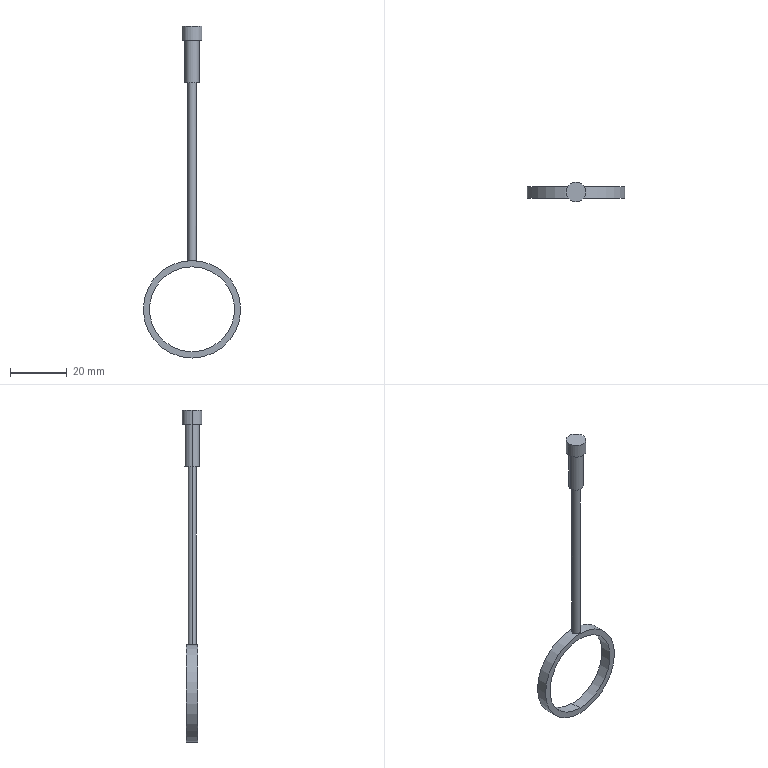Part | STEP file | Resist_ncia- reg. - A | 1 solid | 15 faces | box 34.4 x 7 x 117.2 mm | volume 1821 mm3 | cylinder 10 | plane 5 | commonest cylinder face diameters 3 x2 5 x2 7 x2 30 x2 34.4 x2
STEP:
#1=CARTESIAN_POINT('',(0.,0.,0.));
#2=DIRECTION('',(0.,0.,1.));
#3=DIRECTION('',(1.,0.,0.));
#4=AXIS2_PLACEMENT_3D('',#1,#2,#3);
#5=CARTESIAN_POINT('',(0.,-2.,-2.));
#6=VERTEX_POINT('',#5);
#7=CARTESIAN_POINT('',(0.,2.,-2.));
#8=VERTEX_POINT('',#7);
#9=CARTESIAN_POINT('',(0.,-2.,-2.));
#10=DIRECTION('',(0.,1.,0.));
#11=VECTOR('',#10,1.);
#12=LINE('',#9,#11);
#13=CARTESIAN_POINT('',(0.,-2.,-17.));
#14=DIRECTION('',(0.,1.,0.));
#15=DIRECTION('',(0.,0.,1.));
#16=AXIS2_PLACEMENT_3D('',#13,#14,#15);
#17=CYLINDRICAL_SURFACE('',#16,15.);
#18=CARTESIAN_POINT('',(6.283,0.));
#19=DIRECTION('',(0.,1.));
#20=VECTOR('',#19,1.);
#21=LINE('',#18,#20);
#22=(GEOMETRIC_REPRESENTATION_CONTEXT(2)PARAMETRIC_REPRESENTATION_CONTEXT()REPRESENTATION_CONTEXT('',''));
#23=DEFINITIONAL_REPRESENTATION('',(#21),#22);
#24=PCURVE('',#17,#23);
#25=CARTESIAN_POINT('',(0.,-2.,-17.));
#26=DIRECTION('',(0.,1.,0.));
#27=DIRECTION('',(0.,0.,1.));
#28=AXIS2_PLACEMENT_3D('',#25,#26,#27);
#29=CYLINDRICAL_SURFACE('',#28,15.);
#30=CARTESIAN_POINT('',(0.,0.));
#31=DIRECTION('',(0.,1.));
#32=VECTOR('',#31,1.);
#33=LINE('',#30,#32);
#34=(GEOMETRIC_REPRESENTATION_CONTEXT(2)PARAMETRIC_REPRESENTATION_CONTEXT()REPRESENTATION_CONTEXT('',''));
#35=DEFINITIONAL_REPRESENTATION('',(#33),#34);
#36=PCURVE('',#29,#35);
#37=SURFACE_CURVE('',#12,(#24,#36),.PCURVE_S1.);
#38=EDGE_CURVE('',#6,#8,#37,.T.);
#39=ORIENTED_EDGE('',*,*,#38,.T.);
#40=CARTESIAN_POINT('',(0.,2.,-32.));
#41=VERTEX_POINT('',#40);
#42=CARTESIAN_POINT('',(0.,2.,-17.));
#43=DIRECTION('',(0.,1.,0.));
#44=DIRECTION('',(0.,0.,1.));
#45=AXIS2_PLACEMENT_3D('',#42,#43,#44);
#46=CIRCLE('',#45,15.);
#47=CARTESIAN_POINT('',(0.,4.));
#48=DIRECTION('',(1.,0.));
#49=VECTOR('',#48,1.);
#50=LINE('',#47,#49);
#51=(GEOMETRIC_REPRESENTATION_CONTEXT(2)PARAMETRIC_REPRESENTATION_CONTEXT()REPRESENTATION_CONTEXT('',''));
#52=DEFINITIONAL_REPRESENTATION('',(#50),#51);
#53=PCURVE('',#17,#52);
#54=CARTESIAN_POINT('',(0.,2.,-17.));
#55=DIRECTION('',(0.,1.,0.));
#56=DIRECTION('',(0.,0.,1.));
#57=AXIS2_PLACEMENT_3D('',#54,#55,#56);
#58=PLANE('',#57);
#59=CARTESIAN_POINT('',(0.,0.));
#60=DIRECTION('',(1.,0.));
#61=AXIS2_PLACEMENT_2D('',#59,#60);
#62=CIRCLE('',#61,15.);
#63=(GEOMETRIC_REPRESENTATION_CONTEXT(2)PARAMETRIC_REPRESENTATION_CONTEXT()REPRESENTATION_CONTEXT('',''));
#64=DEFINITIONAL_REPRESENTATION('',(#62),#63);
#65=PCURVE('',#58,#64);
#66=SURFACE_CURVE('',#46,(#53,#65),.PCURVE_S1.);
#67=EDGE_CURVE('',#41,#8,#66,.T.);
#68=ORIENTED_EDGE('',*,*,#67,.F.);
#69=CARTESIAN_POINT('',(0.,-2.,-32.));
#70=VERTEX_POINT('',#69);
#71=CARTESIAN_POINT('',(0.,-2.,-32.));
#72=DIRECTION('',(0.,1.,0.));
#73=VECTOR('',#72,1.);
#74=LINE('',#71,#73);
#75=CARTESIAN_POINT('',(3.142,0.));
#76=DIRECTION('',(0.,1.));
#77=VECTOR('',#76,1.);
#78=LINE('',#75,#77);
#79=(GEOMETRIC_REPRESENTATION_CONTEXT(2)PARAMETRIC_REPRESENTATION_CONTEXT()REPRESENTATION_CONTEXT('',''));
#80=DEFINITIONAL_REPRESENTATION('',(#78),#79);
#81=PCURVE('',#17,#80);
#82=CARTESIAN_POINT('',(3.142,0.));
#83=DIRECTION('',(0.,1.));
#84=VECTOR('',#83,1.);
#85=LINE('',#82,#84);
#86=(GEOMETRIC_REPRESENTATION_CONTEXT(2)PARAMETRIC_REPRESENTATION_CONTEXT()REPRESENTATION_CONTEXT('',''));
#87=DEFINITIONAL_REPRESENTATION('',(#85),#86);
#88=PCURVE('',#29,#87);
#89=SURFACE_CURVE('',#74,(#81,#88),.PCURVE_S1.);
#90=EDGE_CURVE('',#70,#41,#89,.T.);
#91=ORIENTED_EDGE('',*,*,#90,.F.);
#92=CARTESIAN_POINT('',(0.,-2.,-17.));
#93=DIRECTION('',(0.,1.,0.));
#94=DIRECTION('',(0.,0.,1.));
#95=AXIS2_PLACEMENT_3D('',#92,#93,#94);
#96=CIRCLE('',#95,15.);
#97=CARTESIAN_POINT('',(0.,0.));
#98=DIRECTION('',(1.,0.));
#99=VECTOR('',#98,1.);
#100=LINE('',#97,#99);
#101=(GEOMETRIC_REPRESENTATION_CONTEXT(2)PARAMETRIC_REPRESENTATION_CONTEXT()REPRESENTATION_CONTEXT('',''));
#102=DEFINITIONAL_REPRESENTATION('',(#100),#101);
#103=PCURVE('',#17,#102);
#104=CARTESIAN_POINT('',(0.,-2.,-17.));
#105=DIRECTION('',(0.,1.,0.));
#106=DIRECTION('',(0.,0.,1.));
#107=AXIS2_PLACEMENT_3D('',#104,#105,#106);
#108=PLANE('',#107);
#109=CARTESIAN_POINT('',(0.,0.));
#110=DIRECTION('',(1.,0.));
#111=AXIS2_PLACEMENT_2D('',#109,#110);
#112=CIRCLE('',#111,15.);
#113=(GEOMETRIC_REPRESENTATION_CONTEXT(2)PARAMETRIC_REPRESENTATION_CONTEXT()REPRESENTATION_CONTEXT('',''));
#114=DEFINITIONAL_REPRESENTATION('',(#112),#113);
#115=PCURVE('',#108,#114);
#116=SURFACE_CURVE('',#96,(#103,#115),.PCURVE_S1.);
#117=EDGE_CURVE('',#70,#6,#116,.T.);
#118=ORIENTED_EDGE('',*,*,#117,.T.);
#119=EDGE_LOOP('',(#39,#68,#91,#118));
#120=FACE_BOUND('',#119,.F.);
#121=ADVANCED_FACE('',(#120),#17,.F.);
#122=CARTESIAN_POINT('',(0.,-2.,0.2));
#123=VERTEX_POINT('',#122);
#124=CARTESIAN_POINT('',(0.,-2.,-34.2));
#125=VERTEX_POINT('',#124);
#126=CARTESIAN_POINT('',(0.,-2.,-17.));
#127=DIRECTION('',(0.,1.,0.));
#128=DIRECTION('',(0.,0.,1.));
#129=AXIS2_PLACEMENT_3D('',#126,#127,#128);
#130=CIRCLE('',#129,17.2);
#131=CARTESIAN_POINT('',(0.,-2.,-17.));
#132=DIRECTION('',(0.,1.,0.));
#133=DIRECTION('',(0.,0.,1.));
#134=AXIS2_PLACEMENT_3D('',#131,#132,#133);
#135=CYLINDRICAL_SURFACE('',#134,17.2);
#136=CARTESIAN_POINT('',(0.,0.));
#137=DIRECTION('',(1.,0.));
#138=VECTOR('',#137,1.);
#139=LINE('',#136,#138);
#140=(GEOMETRIC_REPRESENTATION_CONTEXT(2)PARAMETRIC_REPRESENTATION_CONTEXT()REPRESENTATION_CONTEXT('',''));
#141=DEFINITIONAL_REPRESENTATION('',(#139),#140);
#142=PCURVE('',#135,#141);
#143=CARTESIAN_POINT('',(0.,0.));
#144=DIRECTION('',(1.,0.));
#145=AXIS2_PLACEMENT_2D('',#143,#144);
#146=CIRCLE('',#145,17.2);
#147=(GEOMETRIC_REPRESENTATION_CONTEXT(2)PARAMETRIC_REPRESENTATION_CONTEXT()REPRESENTATION_CONTEXT('',''));
#148=DEFINITIONAL_REPRESENTATION('',(#146),#147);
#149=PCURVE('',#108,#148);
#150=SURFACE_CURVE('',#130,(#142,#149),.PCURVE_S1.);
#151=EDGE_CURVE('',#123,#125,#150,.T.);
#152=ORIENTED_EDGE('',*,*,#151,.T.);
#153=CARTESIAN_POINT('',(0.,2.,-34.2));
#154=VERTEX_POINT('',#153);
#155=CARTESIAN_POINT('',(0.,-2.,-34.2));
#156=DIRECTION('',(0.,1.,0.));
#157=VECTOR('',#156,1.);
#158=LINE('',#155,#157);
#159=CARTESIAN_POINT('',(3.142,0.));
#160=DIRECTION('',(0.,1.));
#161=VECTOR('',#160,1.);
#162=LINE('',#159,#161);
#163=(GEOMETRIC_REPRESENTATION_CONTEXT(2)PARAMETRIC_REPRESENTATION_CONTEXT()REPRESENTATION_CONTEXT('',''));
#164=DEFINITIONAL_REPRESENTATION('',(#162),#163);
#165=PCURVE('',#135,#164);
#166=CARTESIAN_POINT('',(0.,-2.,-17.));
#167=DIRECTION('',(0.,1.,0.));
#168=DIRECTION('',(0.,0.,1.));
#169=AXIS2_PLACEMENT_3D('',#166,#167,#168);
#170=CYLINDRICAL_SURFACE('',#169,17.2);
#171=CARTESIAN_POINT('',(3.142,0.));
#172=DIRECTION('',(0.,1.));
#173=VECTOR('',#172,1.);
#174=LINE('',#171,#173);
#175=(GEOMETRIC_REPRESENTATION_CONTEXT(2)PARAMETRIC_REPRESENTATION_CONTEXT()REPRESENTATION_CONTEXT('',''));
#176=DEFINITIONAL_REPRESENTATION('',(#174),#175);
#177=PCURVE('',#170,#176);
#178=SURFACE_CURVE('',#158,(#165,#177),.PCURVE_S1.);
#179=EDGE_CURVE('',#125,#154,#178,.T.);
#180=ORIENTED_EDGE('',*,*,#179,.T.);
#181=CARTESIAN_POINT('',(0.,2.,0.2));
#182=VERTEX_POINT('',#181);
#183=CARTESIAN_POINT('',(0.,2.,-17.));
#184=DIRECTION('',(0.,1.,0.));
#185=DIRECTION('',(0.,0.,1.));
#186=AXIS2_PLACEMENT_3D('',#183,#184,#185);
#187=CIRCLE('',#186,17.2);
#188=CARTESIAN_POINT('',(0.,4.));
#189=DIRECTION('',(1.,0.));
#190=VECTOR('',#189,1.);
#191=LINE('',#188,#190);
#192=(GEOMETRIC_REPRESENTATION_CONTEXT(2)PARAMETRIC_REPRESENTATION_CONTEXT()REPRESENTATION_CONTEXT('',''));
#193=DEFINITIONAL_REPRESENTATION('',(#191),#192);
#194=PCURVE('',#135,#193);
#195=CARTESIAN_POINT('',(0.,0.));
#196=DIRECTION('',(1.,0.));
#197=AXIS2_PLACEMENT_2D('',#195,#196);
#198=CIRCLE('',#197,17.2);
#199=(GEOMETRIC_REPRESENTATION_CONTEXT(2)PARAMETRIC_REPRESENTATION_CONTEXT()REPRESENTATION_CONTEXT('',''));
#200=DEFINITIONAL_REPRESENTATION('',(#198),#199);
#201=PCURVE('',#58,#200);
#202=SURFACE_CURVE('',#187,(#194,#201),.PCURVE_S1.);
#203=EDGE_CURVE('',#182,#154,#202,.T.);
#204=ORIENTED_EDGE('',*,*,#203,.F.);
#205=CARTESIAN_POINT('',(0.,1.5,0.2));
#206=VERTEX_POINT('',#205);
#207=CARTESIAN_POINT('',(0.,-2.,0.2));
#208=DIRECTION('',(0.,1.,0.));
#209=VECTOR('',#208,1.);
#210=LINE('',#207,#209);
#211=CARTESIAN_POINT('',(0.,0.));
#212=DIRECTION('',(0.,1.));
#213=VECTOR('',#212,1.);
#214=LINE('',#211,#213);
#215=(GEOMETRIC_REPRESENTATION_CONTEXT(2)PARAMETRIC_REPRESENTATION_CONTEXT()REPRESENTATION_CONTEXT('',''));
#216=DEFINITIONAL_REPRESENTATION('',(#214),#215);
#217=PCURVE('',#135,#216);
#218=CARTESIAN_POINT('',(6.283,0.));
#219=DIRECTION('',(0.,1.));
#220=VECTOR('',#219,1.);
#221=LINE('',#218,#220);
#222=(GEOMETRIC_REPRESENTATION_CONTEXT(2)PARAMETRIC_REPRESENTATION_CONTEXT()REPRESENTATION_CONTEXT('',''));
#223=DEFINITIONAL_REPRESENTATION('',(#221),#222);
#224=PCURVE('',#170,#223);
#225=SURFACE_CURVE('',#210,(#217,#224),.PCURVE_S1.);
#226=EDGE_CURVE('',#206,#182,#225,.T.);
#227=ORIENTED_EDGE('',*,*,#226,.F.);
#228=CARTESIAN_POINT('',(1.5,0.,0.1345));
#229=VERTEX_POINT('',#228);
#230=CARTESIAN_POINT('',(1.5,0.,0.1345));
#231=CARTESIAN_POINT('',(1.5,0.1959,0.1345));
#232=CARTESIAN_POINT('',(1.461,0.3934,0.138));
#233=CARTESIAN_POINT('',(1.311,0.7546,0.1501));
#234=CARTESIAN_POINT('',(1.199,0.922,0.1587));
#235=CARTESIAN_POINT('',(0.9918,1.13,0.1715));
#236=CARTESIAN_POINT('',(0.9147,1.193,0.1759));
#237=CARTESIAN_POINT('',(0.7516,1.302,0.1838));
#238=CARTESIAN_POINT('',(0.6654,1.348,0.1874));
#239=CARTESIAN_POINT('',(0.4838,1.423,0.1934));
#240=CARTESIAN_POINT('',(0.3884,1.452,0.1959));
#241=CARTESIAN_POINT('',(0.1966,1.49,0.1991));
#242=CARTESIAN_POINT('',(0.09911,1.5,0.2));
#243=CARTESIAN_POINT('',(0.,1.5,0.2));
#244=B_SPLINE_CURVE_WITH_KNOTS('',3,(#230,#231,#232,#233,#234,#235,#236,#237,#238,#239,#240,#241,#242,#243),.UNSPECIFIED.,.F.,.F.,(4,2,2,2,2,2,4),(0.004692,0.005279,0.005865,0.006159,0.006452,0.006745,0.007038),.UNSPECIFIED.);
#245=CARTESIAN_POINT('',(0.08732,2.));
#246=CARTESIAN_POINT('',(0.08732,2.018));
#247=CARTESIAN_POINT('',(0.08728,2.053));
#248=CARTESIAN_POINT('',(0.08711,2.107));
#249=CARTESIAN_POINT('',(0.08683,2.16));
#250=CARTESIAN_POINT('',(0.08644,2.213));
#251=CARTESIAN_POINT('',(0.08594,2.266));
#252=CARTESIAN_POINT('',(0.08532,2.319));
#253=CARTESIAN_POINT('',(0.08461,2.371));
#254=CARTESIAN_POINT('',(0.08378,2.423));
#255=CARTESIAN_POINT('',(0.08285,2.474));
#256=CARTESIAN_POINT('',(0.08182,2.524));
#257=CARTESIAN_POINT('',(0.08068,2.574));
#258=CARTESIAN_POINT('',(0.07943,2.623));
#259=CARTESIAN_POINT('',(0.07809,2.671));
#260=CARTESIAN_POINT('',(0.07664,2.719));
#261=CARTESIAN_POINT('',(0.07509,2.765));
#262=CARTESIAN_POINT('',(0.07345,2.811));
#263=CARTESIAN_POINT('',(0.07171,2.855));
#264=CARTESIAN_POINT('',(0.06989,2.899));
#265=CARTESIAN_POINT('',(0.06797,2.941));
#266=CARTESIAN_POINT('',(0.06598,2.982));
#267=CARTESIAN_POINT('',(0.0639,3.022));
#268=CARTESIAN_POINT('',(0.06174,3.061));
#269=CARTESIAN_POINT('',(0.0595,3.098));
#270=CARTESIAN_POINT('',(0.05717,3.134));
#271=CARTESIAN_POINT('',(0.05476,3.168));
#272=CARTESIAN_POINT('',(0.05229,3.201));
#273=CARTESIAN_POINT('',(0.04975,3.233));
#274=CARTESIAN_POINT('',(0.04716,3.262));
#275=CARTESIAN_POINT('',(0.04452,3.29));
#276=CARTESIAN_POINT('',(0.04183,3.317));
#277=CARTESIAN_POINT('',(0.03908,3.341));
#278=CARTESIAN_POINT('',(0.03628,3.364));
#279=CARTESIAN_POINT('',(0.03342,3.386));
#280=CARTESIAN_POINT('',(0.03052,3.406));
#281=CARTESIAN_POINT('',(0.02756,3.423));
#282=CARTESIAN_POINT('',(0.02458,3.44));
#283=CARTESIAN_POINT('',(0.02156,3.454));
#284=CARTESIAN_POINT('',(0.01853,3.466));
#285=CARTESIAN_POINT('',(0.01549,3.476));
#286=CARTESIAN_POINT('',(0.01243,3.485));
#287=CARTESIAN_POINT('',(0.009348,3.492));
#288=CARTESIAN_POINT('',(0.006252,3.496));
#289=CARTESIAN_POINT('',(0.003137,3.499));
#290=CARTESIAN_POINT('',(0.001048,3.5));
#291=CARTESIAN_POINT('',(0.,3.5));
#292=B_SPLINE_CURVE_WITH_KNOTS('',3,(#245,#246,#247,#248,#249,#250,#251,#252,#253,#254,#255,#256,#257,#258,#259,#260,#261,#262,#263,#264,#265,#266,#267,#268,#269,#270,#271,#272,#273,#274,#275,#276,#277,#278,#279,#280,#281,#282,#283,#284,#285,#286,#287,#288,#289,#290,#291),.UNSPECIFIED.,.F.,.F.,(4,1,1,1,1,1,1,1,1,1,1,1,1,1,1,1,1,1,1,1,1,1,1,1,1,1,1,1,1,1,1,1,1,1,1,1,1,1,1,1,1,1,1,1,4),(0.004692,0.004745,0.004799,0.004852,0.004905,0.004959,0.005012,0.005065,0.005119,0.005172,0.005225,0.005279,0.005332,0.005385,0.005439,0.005492,0.005545,0.005599,0.005652,0.005705,0.005759,0.005812,0.005865,0.005919,0.005972,0.006025,0.006079,0.006132,0.006185,0.006239,0.006292,0.006345,0.006399,0.006452,0.006505,0.006559,0.006612,0.006665,0.006718,0.006772,0.006825,0.006878,0.006932,0.006985,0.007038),.QUASI_UNIFORM_KNOTS.);
#293=(GEOMETRIC_REPRESENTATION_CONTEXT(2)PARAMETRIC_REPRESENTATION_CONTEXT()REPRESENTATION_CONTEXT('',''));
#294=DEFINITIONAL_REPRESENTATION('',(#292),#293);
#295=PCURVE('',#135,#294);
#296=CARTESIAN_POINT('',(0.,0.,63.));
#297=DIRECTION('',(0.,0.,-1.));
#298=DIRECTION('',(-1.,0.,0.));
#299=AXIS2_PLACEMENT_3D('',#296,#297,#298);
#300=CYLINDRICAL_SURFACE('',#299,1.5);
#301=CARTESIAN_POINT('',(3.142,62.866));
#302=CARTESIAN_POINT('',(3.13,62.866));
#303=CARTESIAN_POINT('',(3.106,62.865));
#304=CARTESIAN_POINT('',(3.07,62.865));
#305=CARTESIAN_POINT('',(3.035,62.865));
#306=CARTESIAN_POINT('',(2.999,62.864));
#307=CARTESIAN_POINT('',(2.963,62.863));
#308=CARTESIAN_POINT('',(2.927,62.863));
#309=CARTESIAN_POINT('',(2.892,62.862));
#310=CARTESIAN_POINT('',(2.856,62.86));
#311=CARTESIAN_POINT('',(2.82,62.859));
#312=CARTESIAN_POINT('',(2.784,62.858));
#313=CARTESIAN_POINT('',(2.749,62.856));
#314=CARTESIAN_POINT('',(2.713,62.854));
#315=CARTESIAN_POINT('',(2.678,62.852));
#316=CARTESIAN_POINT('',(2.642,62.85));
#317=CARTESIAN_POINT('',(2.606,62.848));
#318=CARTESIAN_POINT('',(2.571,62.846));
#319=CARTESIAN_POINT('',(2.535,62.844));
#320=CARTESIAN_POINT('',(2.499,62.842));
#321=CARTESIAN_POINT('',(2.463,62.84));
#322=CARTESIAN_POINT('',(2.428,62.837));
#323=CARTESIAN_POINT('',(2.392,62.835));
#324=CARTESIAN_POINT('',(2.357,62.833));
#325=CARTESIAN_POINT('',(2.321,62.83));
#326=CARTESIAN_POINT('',(2.285,62.828));
#327=CARTESIAN_POINT('',(2.249,62.826));
#328=CARTESIAN_POINT('',(2.213,62.823));
#329=CARTESIAN_POINT('',(2.177,62.821));
#330=CARTESIAN_POINT('',(2.142,62.819));
#331=CARTESIAN_POINT('',(2.106,62.817));
#332=CARTESIAN_POINT('',(2.071,62.815));
#333=CARTESIAN_POINT('',(2.035,62.813));
#334=CARTESIAN_POINT('',(2.,62.811));
#335=CARTESIAN_POINT('',(1.964,62.81));
#336=CARTESIAN_POINT('',(1.928,62.808));
#337=CARTESIAN_POINT('',(1.892,62.807));
#338=CARTESIAN_POINT('',(1.856,62.805));
#339=CARTESIAN_POINT('',(1.821,62.804));
#340=CARTESIAN_POINT('',(1.785,62.803));
#341=CARTESIAN_POINT('',(1.749,62.802));
#342=CARTESIAN_POINT('',(1.714,62.801));
#343=CARTESIAN_POINT('',(1.678,62.801));
#344=CARTESIAN_POINT('',(1.643,62.8));
#345=CARTESIAN_POINT('',(1.607,62.8));
#346=CARTESIAN_POINT('',(1.583,62.8));
#347=CARTESIAN_POINT('',(1.571,62.8));
#348=B_SPLINE_CURVE_WITH_KNOTS('',3,(#301,#302,#303,#304,#305,#306,#307,#308,#309,#310,#311,#312,#313,#314,#315,#316,#317,#318,#319,#320,#321,#322,#323,#324,#325,#326,#327,#328,#329,#330,#331,#332,#333,#334,#335,#336,#337,#338,#339,#340,#341,#342,#343,#344,#345,#346,#347),.UNSPECIFIED.,.F.,.F.,(4,1,1,1,1,1,1,1,1,1,1,1,1,1,1,1,1,1,1,1,1,1,1,1,1,1,1,1,1,1,1,1,1,1,1,1,1,1,1,1,1,1,1,1,4),(0.004692,0.004745,0.004799,0.004852,0.004905,0.004959,0.005012,0.005065,0.005119,0.005172,0.005225,0.005279,0.005332,0.005385,0.005439,0.005492,0.005545,0.005599,0.005652,0.005705,0.005759,0.005812,0.005865,0.005919,0.005972,0.006025,0.006079,0.006132,0.006185,0.006239,0.006292,0.006345,0.006399,0.006452,0.006505,0.006559,0.006612,0.006665,0.006718,0.006772,0.006825,0.006878,0.006932,0.006985,0.007038),.QUASI_UNIFORM_KNOTS.);
#349=(GEOMETRIC_REPRESENTATION_CONTEXT(2)PARAMETRIC_REPRESENTATION_CONTEXT()REPRESENTATION_CONTEXT('',''));
#350=DEFINITIONAL_REPRESENTATION('',(#348),#349);
#351=PCURVE('',#300,#350);
#352=SURFACE_CURVE('',#244,(#295,#351),.PCURVE_S1.);
#353=EDGE_CURVE('',#229,#206,#352,.T.);
#354=ORIENTED_EDGE('',*,*,#353,.F.);
#355=CARTESIAN_POINT('',(0.,-1.5,0.2));
#356=VERTEX_POINT('',#355);
#357=CARTESIAN_POINT('',(0.,-1.5,0.2));
#358=CARTESIAN_POINT('',(0.09787,-1.5,0.2));
#359=CARTESIAN_POINT('',(0.1973,-1.49,0.1991));
#360=CARTESIAN_POINT('',(0.3896,-1.452,0.1959));
#361=CARTESIAN_POINT('',(0.4831,-1.423,0.1935));
#362=CARTESIAN_POINT('',(0.6648,-1.348,0.1874));
#363=CARTESIAN_POINT('',(0.7525,-1.301,0.1837));
#364=CARTESIAN_POINT('',(0.9149,-1.193,0.1758));
#365=CARTESIAN_POINT('',(0.9907,-1.131,0.1716));
#366=CARTESIAN_POINT('',(1.131,-0.9906,0.1629));
#367=CARTESIAN_POINT('',(1.193,-0.9149,0.1587));
#368=CARTESIAN_POINT('',(1.301,-0.7525,0.1508));
#369=CARTESIAN_POINT('',(1.348,-0.6648,0.1471));
#370=CARTESIAN_POINT('',(1.423,-0.4831,0.141));
#371=CARTESIAN_POINT('',(1.452,-0.3896,0.1386));
#372=CARTESIAN_POINT('',(1.49,-0.1973,0.1353));
#373=CARTESIAN_POINT('',(1.5,-0.0979,0.1345));
#374=CARTESIAN_POINT('',(1.5,0.,0.1345));
#375=B_SPLINE_CURVE_WITH_KNOTS('',3,(#357,#358,#359,#360,#361,#362,#363,#364,#365,#366,#367,#368,#369,#370,#371,#372,#373,#374),.UNSPECIFIED.,.F.,.F.,(4,2,2,2,2,2,2,2,4),(0.002346,0.00264,0.002933,0.003226,0.003519,0.003812,0.004106,0.004399,0.004692),.UNSPECIFIED.);
#376=CARTESIAN_POINT('',(0.,0.5));
#377=CARTESIAN_POINT('',(0.001035,0.5));
#378=CARTESIAN_POINT('',(0.00311,0.5006));
#379=CARTESIAN_POINT('',(0.00623,0.5035));
#380=CARTESIAN_POINT('',(0.009348,0.5084));
#381=CARTESIAN_POINT('',(0.01245,0.5151));
#382=CARTESIAN_POINT('',(0.01554,0.5237));
#383=CARTESIAN_POINT('',(0.01859,0.5341));
#384=CARTESIAN_POINT('',(0.02161,0.5464));
#385=CARTESIAN_POINT('',(0.0246,0.5605));
#386=CARTESIAN_POINT('',(0.02756,0.5765));
#387=CARTESIAN_POINT('',(0.03048,0.5942));
#388=CARTESIAN_POINT('',(0.03338,0.6138));
#389=CARTESIAN_POINT('',(0.03624,0.6353));
#390=CARTESIAN_POINT('',(0.03907,0.6585));
#391=CARTESIAN_POINT('',(0.04184,0.6834));
#392=CARTESIAN_POINT('',(0.04455,0.71));
#393=CARTESIAN_POINT('',(0.0472,0.7382));
#394=CARTESIAN_POINT('',(0.04978,0.7678));
#395=CARTESIAN_POINT('',(0.0523,0.7989));
#396=CARTESIAN_POINT('',(0.05475,0.8316));
#397=CARTESIAN_POINT('',(0.05714,0.8659));
#398=CARTESIAN_POINT('',(0.05946,0.9017));
#399=CARTESIAN_POINT('',(0.06172,0.9391));
#400=CARTESIAN_POINT('',(0.0639,0.9779));
#401=CARTESIAN_POINT('',(0.06599,1.018));
#402=CARTESIAN_POINT('',(0.06798,1.059));
#403=CARTESIAN_POINT('',(0.06989,1.101));
#404=CARTESIAN_POINT('',(0.0717,1.144));
#405=CARTESIAN_POINT('',(0.07343,1.188));
#406=CARTESIAN_POINT('',(0.07507,1.234));
#407=CARTESIAN_POINT('',(0.07662,1.281));
#408=CARTESIAN_POINT('',(0.07807,1.328));
#409=CARTESIAN_POINT('',(0.07943,1.377));
#410=CARTESIAN_POINT('',(0.08068,1.426));
#411=CARTESIAN_POINT('',(0.08182,1.476));
#412=CARTESIAN_POINT('',(0.08286,1.526));
#413=CARTESIAN_POINT('',(0.08379,1.577));
#414=CARTESIAN_POINT('',(0.08461,1.628));
#415=CARTESIAN_POINT('',(0.08533,1.68));
#416=CARTESIAN_POINT('',(0.08594,1.733));
#417=CARTESIAN_POINT('',(0.08644,1.786));
#418=CARTESIAN_POINT('',(0.08683,1.839));
#419=CARTESIAN_POINT('',(0.08711,1.893));
#420=CARTESIAN_POINT('',(0.08728,1.946));
#421=CARTESIAN_POINT('',(0.08732,1.982));
#422=CARTESIAN_POINT('',(0.08732,2.));
#423=B_SPLINE_CURVE_WITH_KNOTS('',3,(#376,#377,#378,#379,#380,#381,#382,#383,#384,#385,#386,#387,#388,#389,#390,#391,#392,#393,#394,#395,#396,#397,#398,#399,#400,#401,#402,#403,#404,#405,#406,#407,#408,#409,#410,#411,#412,#413,#414,#415,#416,#417,#418,#419,#420,#421,#422),.UNSPECIFIED.,.F.,.F.,(4,1,1,1,1,1,1,1,1,1,1,1,1,1,1,1,1,1,1,1,1,1,1,1,1,1,1,1,1,1,1,1,1,1,1,1,1,1,1,1,1,1,1,1,4),(0.002346,0.0024,0.002453,0.002506,0.00256,0.002613,0.002666,0.00272,0.002773,0.002826,0.00288,0.002933,0.002986,0.003039,0.003093,0.003146,0.003199,0.003253,0.003306,0.003359,0.003413,0.003466,0.003519,0.003573,0.003626,0.003679,0.003732,0.003786,0.003839,0.003892,0.003946,0.003999,0.004052,0.004106,0.004159,0.004212,0.004265,0.004319,0.004372,0.004425,0.004479,0.004532,0.004585,0.004639,0.004692),.QUASI_UNIFORM_KNOTS.);
#424=(GEOMETRIC_REPRESENTATION_CONTEXT(2)PARAMETRIC_REPRESENTATION_CONTEXT()REPRESENTATION_CONTEXT('',''));
#425=DEFINITIONAL_REPRESENTATION('',(#423),#424);
#426=PCURVE('',#135,#425);
#427=CARTESIAN_POINT('',(0.,0.,63.));
#428=DIRECTION('',(0.,0.,-1.));
#429=DIRECTION('',(-1.,0.,0.));
#430=AXIS2_PLACEMENT_3D('',#427,#428,#429);
#431=CYLINDRICAL_SURFACE('',#430,1.5);
#432=CARTESIAN_POINT('',(4.712,62.8));
#433=CARTESIAN_POINT('',(4.701,62.8));
#434=CARTESIAN_POINT('',(4.677,62.8));
#435=CARTESIAN_POINT('',(4.641,62.8));
#436=CARTESIAN_POINT('',(4.605,62.801));
#437=CARTESIAN_POINT('',(4.569,62.801));
#438=CARTESIAN_POINT('',(4.533,62.802));
#439=CARTESIAN_POINT('',(4.498,62.803));
#440=CARTESIAN_POINT('',(4.462,62.804));
#441=CARTESIAN_POINT('',(4.427,62.805));
#442=CARTESIAN_POINT('',(4.391,62.807));
#443=CARTESIAN_POINT('',(4.355,62.808));
#444=CARTESIAN_POINT('',(4.32,62.81));
#445=CARTESIAN_POINT('',(4.284,62.811));
#446=CARTESIAN_POINT('',(4.248,62.813));
#447=CARTESIAN_POINT('',(4.212,62.815));
#448=CARTESIAN_POINT('',(4.176,62.817));
#449=CARTESIAN_POINT('',(4.141,62.819));
#450=CARTESIAN_POINT('',(4.105,62.821));
#451=CARTESIAN_POINT('',(4.07,62.823));
#452=CARTESIAN_POINT('',(4.034,62.826));
#453=CARTESIAN_POINT('',(3.999,62.828));
#454=CARTESIAN_POINT('',(3.963,62.83));
#455=CARTESIAN_POINT('',(3.927,62.833));
#456=CARTESIAN_POINT('',(3.891,62.835));
#457=CARTESIAN_POINT('',(3.855,62.837));
#458=CARTESIAN_POINT('',(3.82,62.84));
#459=CARTESIAN_POINT('',(3.784,62.842));
#460=CARTESIAN_POINT('',(3.749,62.844));
#461=CARTESIAN_POINT('',(3.713,62.846));
#462=CARTESIAN_POINT('',(3.677,62.848));
#463=CARTESIAN_POINT('',(3.642,62.85));
#464=CARTESIAN_POINT('',(3.606,62.852));
#465=CARTESIAN_POINT('',(3.57,62.854));
#466=CARTESIAN_POINT('',(3.534,62.856));
#467=CARTESIAN_POINT('',(3.499,62.858));
#468=CARTESIAN_POINT('',(3.463,62.859));
#469=CARTESIAN_POINT('',(3.427,62.86));
#470=CARTESIAN_POINT('',(3.392,62.862));
#471=CARTESIAN_POINT('',(3.356,62.863));
#472=CARTESIAN_POINT('',(3.321,62.863));
#473=CARTESIAN_POINT('',(3.285,62.864));
#474=CARTESIAN_POINT('',(3.249,62.865));
#475=CARTESIAN_POINT('',(3.213,62.865));
#476=CARTESIAN_POINT('',(3.177,62.865));
#477=CARTESIAN_POINT('',(3.153,62.866));
#478=CARTESIAN_POINT('',(3.142,62.866));
#479=B_SPLINE_CURVE_WITH_KNOTS('',3,(#432,#433,#434,#435,#436,#437,#438,#439,#440,#441,#442,#443,#444,#445,#446,#447,#448,#449,#450,#451,#452,#453,#454,#455,#456,#457,#458,#459,#460,#461,#462,#463,#464,#465,#466,#467,#468,#469,#470,#471,#472,#473,#474,#475,#476,#477,#478),.UNSPECIFIED.,.F.,.F.,(4,1,1,1,1,1,1,1,1,1,1,1,1,1,1,1,1,1,1,1,1,1,1,1,1,1,1,1,1,1,1,1,1,1,1,1,1,1,1,1,1,1,1,1,4),(0.002346,0.0024,0.002453,0.002506,0.00256,0.002613,0.002666,0.00272,0.002773,0.002826,0.00288,0.002933,0.002986,0.003039,0.003093,0.003146,0.003199,0.003253,0.003306,0.003359,0.003413,0.003466,0.003519,0.003573,0.003626,0.003679,0.003732,0.003786,0.003839,0.003892,0.003946,0.003999,0.004052,0.004106,0.004159,0.004212,0.004265,0.004319,0.004372,0.004425,0.004479,0.004532,0.004585,0.004639,0.004692),.QUASI_UNIFORM_KNOTS.);
#480=(GEOMETRIC_REPRESENTATION_CONTEXT(2)PARAMETRIC_REPRESENTATION_CONTEXT()REPRESENTATION_CONTEXT('',''));
#481=DEFINITIONAL_REPRESENTATION('',(#479),#480);
#482=PCURVE('',#431,#481);
#483=SURFACE_CURVE('',#375,(#426,#482),.PCURVE_S1.);
#484=EDGE_CURVE('',#356,#229,#483,.T.);
#485=ORIENTED_EDGE('',*,*,#484,.F.);
#486=CARTESIAN_POINT('',(0.,-2.,0.2));
#487=DIRECTION('',(0.,1.,0.));
#488=VECTOR('',#487,1.);
#489=LINE('',#486,#488);
#490=CARTESIAN_POINT('',(0.,0.));
#491=DIRECTION('',(0.,1.));
#492=VECTOR('',#491,1.);
#493=LINE('',#490,#492);
#494=(GEOMETRIC_REPRESENTATION_CONTEXT(2)PARAMETRIC_REPRESENTATION_CONTEXT()REPRESENTATION_CONTEXT('',''));
#495=DEFINITIONAL_REPRESENTATION('',(#493),#494);
#496=PCURVE('',#135,#495);
#497=CARTESIAN_POINT('',(6.283,0.));
#498=DIRECTION('',(0.,1.));
#499=VECTOR('',#498,1.);
#500=LINE('',#497,#499);
#501=(GEOMETRIC_REPRESENTATION_CONTEXT(2)PARAMETRIC_REPRESENTATION_CONTEXT()REPRESENTATION_CONTEXT('',''));
#502=DEFINITIONAL_REPRESENTATION('',(#500),#501);
#503=PCURVE('',#170,#502);
#504=SURFACE_CURVE('',#489,(#496,#503),.PCURVE_S1.);
#505=EDGE_CURVE('',#123,#356,#504,.T.);
#506=ORIENTED_EDGE('',*,*,#505,.F.);
#507=EDGE_LOOP('',(#152,#180,#204,#227,#354,#485,#506));
#508=FACE_BOUND('',#507,.T.);
#509=ADVANCED_FACE('',(#508),#135,.T.);
#510=CARTESIAN_POINT('',(3.5,0.,83.));
#511=VERTEX_POINT('',#510);
#512=CARTESIAN_POINT('',(-3.5,0.,83.));
#513=VERTEX_POINT('',#512);
#514=CARTESIAN_POINT('',(0.,0.,83.));
#515=DIRECTION('',(0.,0.,1.));
#516=DIRECTION('',(1.,0.,0.));
#517=AXIS2_PLACEMENT_3D('',#514,#515,#516);
#518=CIRCLE('',#517,3.5);
#519=CARTESIAN_POINT('',(0.,0.,83.));
#520=DIRECTION('',(0.,0.,-1.));
#521=DIRECTION('',(-1.,0.,0.));
#522=AXIS2_PLACEMENT_3D('',#519,#520,#521);
#523=CYLINDRICAL_SURFACE('',#522,3.5);
#524=CARTESIAN_POINT('',(3.142,0.));
#525=DIRECTION('',(-1.,0.));
#526=VECTOR('',#525,1.);
#527=LINE('',#524,#526);
#528=(GEOMETRIC_REPRESENTATION_CONTEXT(2)PARAMETRIC_REPRESENTATION_CONTEXT()REPRESENTATION_CONTEXT('',''));
#529=DEFINITIONAL_REPRESENTATION('',(#527),#528);
#530=PCURVE('',#523,#529);
#531=CARTESIAN_POINT('',(0.,0.,83.));
#532=DIRECTION('',(0.,0.,1.));
#533=DIRECTION('',(1.,0.,0.));
#534=AXIS2_PLACEMENT_3D('',#531,#532,#533);
#535=PLANE('',#534);
#536=CARTESIAN_POINT('',(0.,0.));
#537=DIRECTION('',(1.,0.));
#538=AXIS2_PLACEMENT_2D('',#536,#537);
#539=CIRCLE('',#538,3.5);
#540=(GEOMETRIC_REPRESENTATION_CONTEXT(2)PARAMETRIC_REPRESENTATION_CONTEXT()REPRESENTATION_CONTEXT('',''));
#541=DEFINITIONAL_REPRESENTATION('',(#539),#540);
#542=PCURVE('',#535,#541);
#543=SURFACE_CURVE('',#518,(#530,#542),.PCURVE_S1.);
#544=EDGE_CURVE('',#511,#513,#543,.T.);
#545=ORIENTED_EDGE('',*,*,#544,.F.);
#546=CARTESIAN_POINT('',(3.5,0.,78.));
#547=VERTEX_POINT('',#546);
#548=CARTESIAN_POINT('',(3.5,0.,83.));
#549=DIRECTION('',(0.,0.,-1.));
#550=VECTOR('',#549,1.);
#551=LINE('',#548,#550);
#552=CARTESIAN_POINT('',(3.142,0.));
#553=DIRECTION('',(0.,1.));
#554=VECTOR('',#553,1.);
#555=LINE('',#552,#554);
#556=(GEOMETRIC_REPRESENTATION_CONTEXT(2)PARAMETRIC_REPRESENTATION_CONTEXT()REPRESENTATION_CONTEXT('',''));
#557=DEFINITIONAL_REPRESENTATION('',(#555),#556);
#558=PCURVE('',#523,#557);
#559=CARTESIAN_POINT('',(0.,0.,83.));
#560=DIRECTION('',(0.,0.,-1.));
#561=DIRECTION('',(-1.,0.,0.));
#562=AXIS2_PLACEMENT_3D('',#559,#560,#561);
#563=CYLINDRICAL_SURFACE('',#562,3.5);
#564=CARTESIAN_POINT('',(3.142,0.));
#565=DIRECTION('',(0.,1.));
#566=VECTOR('',#565,1.);
#567=LINE('',#564,#566);
#568=(GEOMETRIC_REPRESENTATION_CONTEXT(2)PARAMETRIC_REPRESENTATION_CONTEXT()REPRESENTATION_CONTEXT('',''));
#569=DEFINITIONAL_REPRESENTATION('',(#567),#568);
#570=PCURVE('',#563,#569);
#571=SURFACE_CURVE('',#551,(#558,#570),.PCURVE_S1.);
#572=EDGE_CURVE('',#511,#547,#571,.T.);
#573=ORIENTED_EDGE('',*,*,#572,.T.);
#574=CARTESIAN_POINT('',(-3.5,0.,78.));
#575=VERTEX_POINT('',#574);
#576=CARTESIAN_POINT('',(0.,0.,78.));
#577=DIRECTION('',(0.,0.,1.));
#578=DIRECTION('',(1.,0.,0.));
#579=AXIS2_PLACEMENT_3D('',#576,#577,#578);
#580=CIRCLE('',#579,3.5);
#581=CARTESIAN_POINT('',(3.142,5.));
#582=DIRECTION('',(-1.,0.));
#583=VECTOR('',#582,1.);
#584=LINE('',#581,#583);
#585=(GEOMETRIC_REPRESENTATION_CONTEXT(2)PARAMETRIC_REPRESENTATION_CONTEXT()REPRESENTATION_CONTEXT('',''));
#586=DEFINITIONAL_REPRESENTATION('',(#584),#585);
#587=PCURVE('',#523,#586);
#588=CARTESIAN_POINT('',(0.,0.,78.));
#589=DIRECTION('',(0.,0.,1.));
#590=DIRECTION('',(1.,0.,0.));
#591=AXIS2_PLACEMENT_3D('',#588,#589,#590);
#592=PLANE('',#591);
#593=CARTESIAN_POINT('',(0.,0.));
#594=DIRECTION('',(1.,0.));
#595=AXIS2_PLACEMENT_2D('',#593,#594);
#596=CIRCLE('',#595,3.5);
#597=(GEOMETRIC_REPRESENTATION_CONTEXT(2)PARAMETRIC_REPRESENTATION_CONTEXT()REPRESENTATION_CONTEXT('',''));
#598=DEFINITIONAL_REPRESENTATION('',(#596),#597);
#599=PCURVE('',#592,#598);
#600=SURFACE_CURVE('',#580,(#587,#599),.PCURVE_S1.);
#601=EDGE_CURVE('',#547,#575,#600,.T.);
#602=ORIENTED_EDGE('',*,*,#601,.T.);
#603=CARTESIAN_POINT('',(-3.5,0.,83.));
#604=DIRECTION('',(0.,0.,-1.));
#605=VECTOR('',#604,1.);
#606=LINE('',#603,#605);
#607=CARTESIAN_POINT('',(0.,0.));
#608=DIRECTION('',(0.,1.));
#609=VECTOR('',#608,1.);
#610=LINE('',#607,#609);
#611=(GEOMETRIC_REPRESENTATION_CONTEXT(2)PARAMETRIC_REPRESENTATION_CONTEXT()REPRESENTATION_CONTEXT('',''));
#612=DEFINITIONAL_REPRESENTATION('',(#610),#611);
#613=PCURVE('',#523,#612);
#614=CARTESIAN_POINT('',(6.283,0.));
#615=DIRECTION('',(0.,1.));
#616=VECTOR('',#615,1.);
#617=LINE('',#614,#616);
#618=(GEOMETRIC_REPRESENTATION_CONTEXT(2)PARAMETRIC_REPRESENTATION_CONTEXT()REPRESENTATION_CONTEXT('',''));
#619=DEFINITIONAL_REPRESENTATION('',(#617),#618);
#620=PCURVE('',#563,#619);
#621=SURFACE_CURVE('',#606,(#613,#620),.PCURVE_S1.);
#622=EDGE_CURVE('',#513,#575,#621,.T.);
#623=ORIENTED_EDGE('',*,*,#622,.F.);
#624=EDGE_LOOP('',(#545,#573,#602,#623));
#625=FACE_BOUND('',#624,.T.);
#626=ADVANCED_FACE('',(#625),#523,.T.);
#627=CARTESIAN_POINT('',(2.5,0.,78.));
#628=VERTEX_POINT('',#627);
#629=CARTESIAN_POINT('',(-2.5,0.,78.));
#630=VERTEX_POINT('',#629);
#631=CARTESIAN_POINT('',(0.,0.,78.));
#632=DIRECTION('',(0.,0.,1.));
#633=DIRECTION('',(1.,0.,0.));
#634=AXIS2_PLACEMENT_3D('',#631,#632,#633);
#635=CIRCLE('',#634,2.5);
#636=CARTESIAN_POINT('',(0.,0.,78.));
#637=DIRECTION('',(0.,0.,-1.));
#638=DIRECTION('',(-1.,0.,0.));
#639=AXIS2_PLACEMENT_3D('',#636,#637,#638);
#640=CYLINDRICAL_SURFACE('',#639,2.5);
#641=CARTESIAN_POINT('',(3.142,0.));
#642=DIRECTION('',(-1.,0.));
#643=VECTOR('',#642,1.);
#644=LINE('',#641,#643);
#645=(GEOMETRIC_REPRESENTATION_CONTEXT(2)PARAMETRIC_REPRESENTATION_CONTEXT()REPRESENTATION_CONTEXT('',''));
#646=DEFINITIONAL_REPRESENTATION('',(#644),#645);
#647=PCURVE('',#640,#646);
#648=CARTESIAN_POINT('',(0.,0.));
#649=DIRECTION('',(1.,0.));
#650=AXIS2_PLACEMENT_2D('',#648,#649);
#651=CIRCLE('',#650,2.5);
#652=(GEOMETRIC_REPRESENTATION_CONTEXT(2)PARAMETRIC_REPRESENTATION_CONTEXT()REPRESENTATION_CONTEXT('',''));
#653=DEFINITIONAL_REPRESENTATION('',(#651),#652);
#654=PCURVE('',#592,#653);
#655=SURFACE_CURVE('',#635,(#647,#654),.PCURVE_S1.);
#656=EDGE_CURVE('',#628,#630,#655,.T.);
#657=ORIENTED_EDGE('',*,*,#656,.F.);
#658=CARTESIAN_POINT('',(2.5,0.,63.));
#659=VERTEX_POINT('',#658);
#660=CARTESIAN_POINT('',(2.5,0.,78.));
#661=DIRECTION('',(0.,0.,-1.));
#662=VECTOR('',#661,1.);
#663=LINE('',#660,#662);
#664=CARTESIAN_POINT('',(3.142,0.));
#665=DIRECTION('',(0.,1.));
#666=VECTOR('',#665,1.);
#667=LINE('',#664,#666);
#668=(GEOMETRIC_REPRESENTATION_CONTEXT(2)PARAMETRIC_REPRESENTATION_CONTEXT()REPRESENTATION_CONTEXT('',''));
#669=DEFINITIONAL_REPRESENTATION('',(#667),#668);
#670=PCURVE('',#640,#669);
#671=CARTESIAN_POINT('',(0.,0.,78.));
#672=DIRECTION('',(0.,0.,-1.));
#673=DIRECTION('',(-1.,0.,0.));
#674=AXIS2_PLACEMENT_3D('',#671,#672,#673);
#675=CYLINDRICAL_SURFACE('',#674,2.5);
#676=CARTESIAN_POINT('',(3.142,0.));
#677=DIRECTION('',(0.,1.));
#678=VECTOR('',#677,1.);
#679=LINE('',#676,#678);
#680=(GEOMETRIC_REPRESENTATION_CONTEXT(2)PARAMETRIC_REPRESENTATION_CONTEXT()REPRESENTATION_CONTEXT('',''));
#681=DEFINITIONAL_REPRESENTATION('',(#679),#680);
#682=PCURVE('',#675,#681);
#683=SURFACE_CURVE('',#663,(#670,#682),.PCURVE_S1.);
#684=EDGE_CURVE('',#628,#659,#683,.T.);
#685=ORIENTED_EDGE('',*,*,#684,.T.);
#686=CARTESIAN_POINT('',(-2.5,0.,63.));
#687=VERTEX_POINT('',#686);
#688=CARTESIAN_POINT('',(0.,0.,63.));
#689=DIRECTION('',(0.,0.,1.));
#690=DIRECTION('',(1.,0.,0.));
#691=AXIS2_PLACEMENT_3D('',#688,#689,#690);
#692=CIRCLE('',#691,2.5);
#693=CARTESIAN_POINT('',(3.142,15.));
#694=DIRECTION('',(-1.,0.));
#695=VECTOR('',#694,1.);
#696=LINE('',#693,#695);
#697=(GEOMETRIC_REPRESENTATION_CONTEXT(2)PARAMETRIC_REPRESENTATION_CONTEXT()REPRESENTATION_CONTEXT('',''));
#698=DEFINITIONAL_REPRESENTATION('',(#696),#697);
#699=PCURVE('',#640,#698);
#700=CARTESIAN_POINT('',(0.,0.,63.));
#701=DIRECTION('',(0.,0.,1.));
#702=DIRECTION('',(1.,0.,0.));
#703=AXIS2_PLACEMENT_3D('',#700,#701,#702);
#704=PLANE('',#703);
#705=CARTESIAN_POINT('',(0.,0.));
#706=DIRECTION('',(1.,0.));
#707=AXIS2_PLACEMENT_2D('',#705,#706);
#708=CIRCLE('',#707,2.5);
#709=(GEOMETRIC_REPRESENTATION_CONTEXT(2)PARAMETRIC_REPRESENTATION_CONTEXT()REPRESENTATION_CONTEXT('',''));
#710=DEFINITIONAL_REPRESENTATION('',(#708),#709);
#711=PCURVE('',#704,#710);
#712=SURFACE_CURVE('',#692,(#699,#711),.PCURVE_S1.);
#713=EDGE_CURVE('',#659,#687,#712,.T.);
#714=ORIENTED_EDGE('',*,*,#713,.T.);
#715=CARTESIAN_POINT('',(-2.5,0.,78.));
#716=DIRECTION('',(0.,0.,-1.));
#717=VECTOR('',#716,1.);
#718=LINE('',#715,#717);
#719=CARTESIAN_POINT('',(0.,0.));
#720=DIRECTION('',(0.,1.));
#721=VECTOR('',#720,1.);
#722=LINE('',#719,#721);
#723=(GEOMETRIC_REPRESENTATION_CONTEXT(2)PARAMETRIC_REPRESENTATION_CONTEXT()REPRESENTATION_CONTEXT('',''));
#724=DEFINITIONAL_REPRESENTATION('',(#722),#723);
#725=PCURVE('',#640,#724);
#726=CARTESIAN_POINT('',(6.283,0.));
#727=DIRECTION('',(0.,1.));
#728=VECTOR('',#727,1.);
#729=LINE('',#726,#728);
#730=(GEOMETRIC_REPRESENTATION_CONTEXT(2)PARAMETRIC_REPRESENTATION_CONTEXT()REPRESENTATION_CONTEXT('',''));
#731=DEFINITIONAL_REPRESENTATION('',(#729),#730);
#732=PCURVE('',#675,#731);
#733=SURFACE_CURVE('',#718,(#725,#732),.PCURVE_S1.);
#734=EDGE_CURVE('',#630,#687,#733,.T.);
#735=ORIENTED_EDGE('',*,*,#734,.F.);
#736=EDGE_LOOP('',(#657,#685,#714,#735));
#737=FACE_BOUND('',#736,.T.);
#738=ADVANCED_FACE('',(#737),#640,.T.);
#739=CARTESIAN_POINT('',(1.5,0.,63.));
#740=VERTEX_POINT('',#739);
#741=CARTESIAN_POINT('',(-1.5,0.,63.));
#742=VERTEX_POINT('',#741);
#743=CARTESIAN_POINT('',(0.,0.,63.));
#744=DIRECTION('',(0.,0.,1.));
#745=DIRECTION('',(1.,0.,0.));
#746=AXIS2_PLACEMENT_3D('',#743,#744,#745);
#747=CIRCLE('',#746,1.5);
#748=CARTESIAN_POINT('',(3.142,0.));
#749=DIRECTION('',(-1.,0.));
#750=VECTOR('',#749,1.);
#751=LINE('',#748,#750);
#752=(GEOMETRIC_REPRESENTATION_CONTEXT(2)PARAMETRIC_REPRESENTATION_CONTEXT()REPRESENTATION_CONTEXT('',''));
#753=DEFINITIONAL_REPRESENTATION('',(#751),#752);
#754=PCURVE('',#300,#753);
#755=CARTESIAN_POINT('',(0.,0.));
#756=DIRECTION('',(1.,0.));
#757=AXIS2_PLACEMENT_2D('',#755,#756);
#758=CIRCLE('',#757,1.5);
#759=(GEOMETRIC_REPRESENTATION_CONTEXT(2)PARAMETRIC_REPRESENTATION_CONTEXT()REPRESENTATION_CONTEXT('',''));
#760=DEFINITIONAL_REPRESENTATION('',(#758),#759);
#761=PCURVE('',#704,#760);
#762=SURFACE_CURVE('',#747,(#754,#761),.PCURVE_S1.);
#763=EDGE_CURVE('',#740,#742,#762,.T.);
#764=ORIENTED_EDGE('',*,*,#763,.F.);
#765=CARTESIAN_POINT('',(1.5,0.,63.));
#766=DIRECTION('',(0.,0.,-1.));
#767=VECTOR('',#766,1.);
#768=LINE('',#765,#767);
#769=CARTESIAN_POINT('',(3.142,0.));
#770=DIRECTION('',(0.,1.));
#771=VECTOR('',#770,1.);
#772=LINE('',#769,#771);
#773=(GEOMETRIC_REPRESENTATION_CONTEXT(2)PARAMETRIC_REPRESENTATION_CONTEXT()REPRESENTATION_CONTEXT('',''));
#774=DEFINITIONAL_REPRESENTATION('',(#772),#773);
#775=PCURVE('',#300,#774);
#776=CARTESIAN_POINT('',(3.142,0.));
#777=DIRECTION('',(0.,1.));
#778=VECTOR('',#777,1.);
#779=LINE('',#776,#778);
#780=(GEOMETRIC_REPRESENTATION_CONTEXT(2)PARAMETRIC_REPRESENTATION_CONTEXT()REPRESENTATION_CONTEXT('',''));
#781=DEFINITIONAL_REPRESENTATION('',(#779),#780);
#782=PCURVE('',#431,#781);
#783=SURFACE_CURVE('',#768,(#775,#782),.PCURVE_S1.);
#784=EDGE_CURVE('',#740,#229,#783,.T.);
#785=ORIENTED_EDGE('',*,*,#784,.T.);
#786=ORIENTED_EDGE('',*,*,#353,.T.);
#787=CARTESIAN_POINT('',(-1.5,0.,0.1345));
#788=VERTEX_POINT('',#787);
#789=CARTESIAN_POINT('',(0.,1.5,0.2));
#790=CARTESIAN_POINT('',(-0.198,1.5,0.2));
#791=CARTESIAN_POINT('',(-0.3926,1.461,0.1965));
#792=CARTESIAN_POINT('',(-0.665,1.348,0.1874));
#793=CARTESIAN_POINT('',(-0.7511,1.302,0.1838));
#794=CARTESIAN_POINT('',(-0.914,1.193,0.1759));
#795=CARTESIAN_POINT('',(-0.9912,1.13,0.1716));
#796=CARTESIAN_POINT('',(-1.199,0.9228,0.1587));
#797=CARTESIAN_POINT('',(-1.31,0.7557,0.1502));
#798=CARTESIAN_POINT('',(-1.46,0.3951,0.1381));
#799=CARTESIAN_POINT('',(-1.5,0.1982,0.1345));
#800=CARTESIAN_POINT('',(-1.5,0.,0.1345));
#801=B_SPLINE_CURVE_WITH_KNOTS('',3,(#789,#790,#791,#792,#793,#794,#795,#796,#797,#798,#799,#800),.UNSPECIFIED.,.F.,.F.,(4,2,2,2,2,4),(0.007038,0.007625,0.007918,0.008211,0.008797,0.009383),.UNSPECIFIED.);
#802=CARTESIAN_POINT('',(1.571,62.8));
#803=CARTESIAN_POINT('',(1.547,62.8));
#804=CARTESIAN_POINT('',(1.499,62.8));
#805=CARTESIAN_POINT('',(1.427,62.801));
#806=CARTESIAN_POINT('',(1.356,62.803));
#807=CARTESIAN_POINT('',(1.285,62.805));
#808=CARTESIAN_POINT('',(1.214,62.808));
#809=CARTESIAN_POINT('',(1.142,62.811));
#810=CARTESIAN_POINT('',(1.071,62.815));
#811=CARTESIAN_POINT('',(1.,62.819));
#812=CARTESIAN_POINT('',(0.9289,62.823));
#813=CARTESIAN_POINT('',(0.8571,62.828));
#814=CARTESIAN_POINT('',(0.7857,62.833));
#815=CARTESIAN_POINT('',(0.7146,62.837));
#816=CARTESIAN_POINT('',(0.6432,62.842));
#817=CARTESIAN_POINT('',(0.5718,62.846));
#818=CARTESIAN_POINT('',(0.5004,62.85));
#819=CARTESIAN_POINT('',(0.4292,62.854));
#820=CARTESIAN_POINT('',(0.3582,62.858));
#821=CARTESIAN_POINT('',(0.2869,62.86));
#822=CARTESIAN_POINT('',(0.2155,62.863));
#823=CARTESIAN_POINT('',(0.1438,62.864));
#824=CARTESIAN_POINT('',(0.07201,62.865));
#825=CARTESIAN_POINT('',(0.02402,62.866));
#826=CARTESIAN_POINT('',(0.,62.866));
#827=B_SPLINE_CURVE_WITH_KNOTS('',3,(#802,#803,#804,#805,#806,#807,#808,#809,#810,#811,#812,#813,#814,#815,#816,#817,#818,#819,#820,#821,#822,#823,#824,#825,#826),.UNSPECIFIED.,.F.,.F.,(4,1,1,1,1,1,1,1,1,1,1,1,1,1,1,1,1,1,1,1,1,1,4),(0.007038,0.007145,0.007252,0.007358,0.007465,0.007571,0.007678,0.007784,0.007891,0.007997,0.008104,0.008211,0.008317,0.008424,0.00853,0.008637,0.008743,0.00885,0.008957,0.009063,0.00917,0.009276,0.009383),.QUASI_UNIFORM_KNOTS.);
#828=(GEOMETRIC_REPRESENTATION_CONTEXT(2)PARAMETRIC_REPRESENTATION_CONTEXT()REPRESENTATION_CONTEXT('',''));
#829=DEFINITIONAL_REPRESENTATION('',(#827),#828);
#830=PCURVE('',#300,#829);
#831=CARTESIAN_POINT('',(6.283,3.5));
#832=CARTESIAN_POINT('',(6.281,3.5));
#833=CARTESIAN_POINT('',(6.277,3.497));
#834=CARTESIAN_POINT('',(6.271,3.486));
#835=CARTESIAN_POINT('',(6.265,3.467));
#836=CARTESIAN_POINT('',(6.259,3.44));
#837=CARTESIAN_POINT('',(6.253,3.407));
#838=CARTESIAN_POINT('',(6.247,3.365));
#839=CARTESIAN_POINT('',(6.241,3.318));
#840=CARTESIAN_POINT('',(6.236,3.263));
#841=CARTESIAN_POINT('',(6.231,3.202));
#842=CARTESIAN_POINT('',(6.226,3.135));
#843=CARTESIAN_POINT('',(6.221,3.062));
#844=CARTESIAN_POINT('',(6.217,2.984));
#845=CARTESIAN_POINT('',(6.213,2.9));
#846=CARTESIAN_POINT('',(6.21,2.812));
#847=CARTESIAN_POINT('',(6.207,2.72));
#848=CARTESIAN_POINT('',(6.204,2.625));
#849=CARTESIAN_POINT('',(6.201,2.526));
#850=CARTESIAN_POINT('',(6.199,2.425));
#851=CARTESIAN_POINT('',(6.198,2.321));
#852=CARTESIAN_POINT('',(6.197,2.215));
#853=CARTESIAN_POINT('',(6.196,2.108));
#854=CARTESIAN_POINT('',(6.196,2.036));
#855=CARTESIAN_POINT('',(6.196,2.));
#856=B_SPLINE_CURVE_WITH_KNOTS('',3,(#831,#832,#833,#834,#835,#836,#837,#838,#839,#840,#841,#842,#843,#844,#845,#846,#847,#848,#849,#850,#851,#852,#853,#854,#855),.UNSPECIFIED.,.F.,.F.,(4,1,1,1,1,1,1,1,1,1,1,1,1,1,1,1,1,1,1,1,1,1,4),(0.007038,0.007145,0.007252,0.007358,0.007465,0.007571,0.007678,0.007784,0.007891,0.007997,0.008104,0.008211,0.008317,0.008424,0.00853,0.008637,0.008743,0.00885,0.008957,0.009063,0.00917,0.009276,0.009383),.QUASI_UNIFORM_KNOTS.);
#857=(GEOMETRIC_REPRESENTATION_CONTEXT(2)PARAMETRIC_REPRESENTATION_CONTEXT()REPRESENTATION_CONTEXT('',''));
#858=DEFINITIONAL_REPRESENTATION('',(#856),#857);
#859=PCURVE('',#170,#858);
#860=SURFACE_CURVE('',#801,(#830,#859),.PCURVE_S1.);
#861=EDGE_CURVE('',#206,#788,#860,.T.);
#862=ORIENTED_EDGE('',*,*,#861,.T.);
#863=CARTESIAN_POINT('',(-1.5,0.,63.));
#864=DIRECTION('',(0.,0.,-1.));
#865=VECTOR('',#864,1.);
#866=LINE('',#863,#865);
#867=CARTESIAN_POINT('',(0.,0.));
#868=DIRECTION('',(0.,1.));
#869=VECTOR('',#868,1.);
#870=LINE('',#867,#869);
#871=(GEOMETRIC_REPRESENTATION_CONTEXT(2)PARAMETRIC_REPRESENTATION_CONTEXT()REPRESENTATION_CONTEXT('',''));
#872=DEFINITIONAL_REPRESENTATION('',(#870),#871);
#873=PCURVE('',#300,#872);
#874=CARTESIAN_POINT('',(6.283,0.));
#875=DIRECTION('',(0.,1.));
#876=VECTOR('',#875,1.);
#877=LINE('',#874,#876);
#878=(GEOMETRIC_REPRESENTATION_CONTEXT(2)PARAMETRIC_REPRESENTATION_CONTEXT()REPRESENTATION_CONTEXT('',''));
#879=DEFINITIONAL_REPRESENTATION('',(#877),#878);
#880=PCURVE('',#431,#879);
#881=SURFACE_CURVE('',#866,(#873,#880),.PCURVE_S1.);
#882=EDGE_CURVE('',#742,#788,#881,.T.);
#883=ORIENTED_EDGE('',*,*,#882,.F.);
#884=EDGE_LOOP('',(#764,#785,#786,#862,#883));
#885=FACE_BOUND('',#884,.T.);
#886=ADVANCED_FACE('',(#885),#300,.T.);
#887=ORIENTED_EDGE('',*,*,#784,.F.);
#888=CARTESIAN_POINT('',(0.,0.,63.));
#889=DIRECTION('',(0.,0.,1.));
#890=DIRECTION('',(1.,0.,0.));
#891=AXIS2_PLACEMENT_3D('',#888,#889,#890);
#892=CIRCLE('',#891,1.5);
#893=CARTESIAN_POINT('',(9.425,0.));
#894=DIRECTION('',(-1.,0.));
#895=VECTOR('',#894,1.);
#896=LINE('',#893,#895);
#897=(GEOMETRIC_REPRESENTATION_CONTEXT(2)PARAMETRIC_REPRESENTATION_CONTEXT()REPRESENTATION_CONTEXT('',''));
#898=DEFINITIONAL_REPRESENTATION('',(#896),#897);
#899=PCURVE('',#431,#898);
#900=CARTESIAN_POINT('',(0.,0.));
#901=DIRECTION('',(1.,0.));
#902=AXIS2_PLACEMENT_2D('',#900,#901);
#903=CIRCLE('',#902,1.5);
#904=(GEOMETRIC_REPRESENTATION_CONTEXT(2)PARAMETRIC_REPRESENTATION_CONTEXT()REPRESENTATION_CONTEXT('',''));
#905=DEFINITIONAL_REPRESENTATION('',(#903),#904);
#906=PCURVE('',#704,#905);
#907=SURFACE_CURVE('',#892,(#899,#906),.PCURVE_S1.);
#908=EDGE_CURVE('',#742,#740,#907,.T.);
#909=ORIENTED_EDGE('',*,*,#908,.F.);
#910=ORIENTED_EDGE('',*,*,#882,.T.);
#911=CARTESIAN_POINT('',(-1.5,0.,0.1345));
#912=CARTESIAN_POINT('',(-1.5,-0.09918,0.1345));
#913=CARTESIAN_POINT('',(-1.49,-0.1967,0.1353));
#914=CARTESIAN_POINT('',(-1.452,-0.3885,0.1386));
#915=CARTESIAN_POINT('',(-1.423,-0.4838,0.1411));
#916=CARTESIAN_POINT('',(-1.348,-0.6655,0.1471));
#917=CARTESIAN_POINT('',(-1.302,-0.7517,0.1508));
#918=CARTESIAN_POINT('',(-1.193,-0.9147,0.1587));
#919=CARTESIAN_POINT('',(-1.129,-0.9919,0.163));
#920=CARTESIAN_POINT('',(-0.9219,-1.199,0.1758));
#921=CARTESIAN_POINT('',(-0.7545,-1.311,0.1844));
#922=CARTESIAN_POINT('',(-0.3934,-1.461,0.1965));
#923=CARTESIAN_POINT('',(-0.1958,-1.5,0.2));
#924=CARTESIAN_POINT('',(0.,-1.5,0.2));
#925=B_SPLINE_CURVE_WITH_KNOTS('',3,(#911,#912,#913,#914,#915,#916,#917,#918,#919,#920,#921,#922,#923,#924),.UNSPECIFIED.,.F.,.F.,(4,2,2,2,2,2,4),(0.,0.0002933,0.0005866,0.0008799,0.001173,0.00176,0.002346),.UNSPECIFIED.);
#926=CARTESIAN_POINT('',(6.283,62.866));
#927=CARTESIAN_POINT('',(6.271,62.866));
#928=CARTESIAN_POINT('',(6.247,62.865));
#929=CARTESIAN_POINT('',(6.211,62.865));
#930=CARTESIAN_POINT('',(6.176,62.865));
#931=CARTESIAN_POINT('',(6.14,62.864));
#932=CARTESIAN_POINT('',(6.105,62.863));
#933=CARTESIAN_POINT('',(6.069,62.863));
#934=CARTESIAN_POINT('',(6.033,62.862));
#935=CARTESIAN_POINT('',(5.998,62.86));
#936=CARTESIAN_POINT('',(5.962,62.859));
#937=CARTESIAN_POINT('',(5.926,62.858));
#938=CARTESIAN_POINT('',(5.89,62.856));
#939=CARTESIAN_POINT('',(5.854,62.854));
#940=CARTESIAN_POINT('',(5.819,62.852));
#941=CARTESIAN_POINT('',(5.783,62.85));
#942=CARTESIAN_POINT('',(5.748,62.848));
#943=CARTESIAN_POINT('',(5.712,62.846));
#944=CARTESIAN_POINT('',(5.676,62.844));
#945=CARTESIAN_POINT('',(5.641,62.842));
#946=CARTESIAN_POINT('',(5.605,62.84));
#947=CARTESIAN_POINT('',(5.569,62.837));
#948=CARTESIAN_POINT('',(5.533,62.835));
#949=CARTESIAN_POINT('',(5.497,62.833));
#950=CARTESIAN_POINT('',(5.462,62.83));
#951=CARTESIAN_POINT('',(5.426,62.828));
#952=CARTESIAN_POINT('',(5.39,62.826));
#953=CARTESIAN_POINT('',(5.355,62.823));
#954=CARTESIAN_POINT('',(5.319,62.821));
#955=CARTESIAN_POINT('',(5.283,62.819));
#956=CARTESIAN_POINT('',(5.248,62.817));
#957=CARTESIAN_POINT('',(5.212,62.815));
#958=CARTESIAN_POINT('',(5.176,62.813));
#959=CARTESIAN_POINT('',(5.141,62.811));
#960=CARTESIAN_POINT('',(5.105,62.81));
#961=CARTESIAN_POINT('',(5.069,62.808));
#962=CARTESIAN_POINT('',(5.034,62.807));
#963=CARTESIAN_POINT('',(4.998,62.805));
#964=CARTESIAN_POINT('',(4.962,62.804));
#965=CARTESIAN_POINT('',(4.927,62.803));
#966=CARTESIAN_POINT('',(4.891,62.802));
#967=CARTESIAN_POINT('',(4.855,62.801));
#968=CARTESIAN_POINT('',(4.819,62.801));
#969=CARTESIAN_POINT('',(4.784,62.8));
#970=CARTESIAN_POINT('',(4.748,62.8));
#971=CARTESIAN_POINT('',(4.724,62.8));
#972=CARTESIAN_POINT('',(4.712,62.8));
#973=B_SPLINE_CURVE_WITH_KNOTS('',3,(#926,#927,#928,#929,#930,#931,#932,#933,#934,#935,#936,#937,#938,#939,#940,#941,#942,#943,#944,#945,#946,#947,#948,#949,#950,#951,#952,#953,#954,#955,#956,#957,#958,#959,#960,#961,#962,#963,#964,#965,#966,#967,#968,#969,#970,#971,#972),.UNSPECIFIED.,.F.,.F.,(4,1,1,1,1,1,1,1,1,1,1,1,1,1,1,1,1,1,1,1,1,1,1,1,1,1,1,1,1,1,1,1,1,1,1,1,1,1,1,1,1,1,1,1,4),(0.,0.00005333,0.0001067,0.00016,0.0002133,0.0002666,0.00032,0.0003733,0.0004266,0.00048,0.0005333,0.0005866,0.00064,0.0006933,0.0007466,0.0007999,0.0008533,0.0009066,0.0009599,0.001013,0.001067,0.00112,0.001173,0.001227,0.00128,0.001333,0.001387,0.00144,0.001493,0.001547,0.0016,0.001653,0.001707,0.00176,0.001813,0.001867,0.00192,0.001973,0.002027,0.00208,0.002133,0.002187,0.00224,0.002293,0.002346),.QUASI_UNIFORM_KNOTS.);
#974=(GEOMETRIC_REPRESENTATION_CONTEXT(2)PARAMETRIC_REPRESENTATION_CONTEXT()REPRESENTATION_CONTEXT('',''));
#975=DEFINITIONAL_REPRESENTATION('',(#973),#974);
#976=PCURVE('',#431,#975);
#977=CARTESIAN_POINT('',(6.196,2.));
#978=CARTESIAN_POINT('',(6.196,1.982));
#979=CARTESIAN_POINT('',(6.196,1.946));
#980=CARTESIAN_POINT('',(6.196,1.892));
#981=CARTESIAN_POINT('',(6.196,1.839));
#982=CARTESIAN_POINT('',(6.197,1.786));
#983=CARTESIAN_POINT('',(6.197,1.734));
#984=CARTESIAN_POINT('',(6.198,1.681));
#985=CARTESIAN_POINT('',(6.199,1.629));
#986=CARTESIAN_POINT('',(6.199,1.577));
#987=CARTESIAN_POINT('',(6.2,1.526));
#988=CARTESIAN_POINT('',(6.201,1.475));
#989=CARTESIAN_POINT('',(6.203,1.425));
#990=CARTESIAN_POINT('',(6.204,1.376));
#991=CARTESIAN_POINT('',(6.205,1.328));
#992=CARTESIAN_POINT('',(6.207,1.281));
#993=CARTESIAN_POINT('',(6.208,1.234));
#994=CARTESIAN_POINT('',(6.21,1.189));
#995=CARTESIAN_POINT('',(6.211,1.145));
#996=CARTESIAN_POINT('',(6.213,1.101));
#997=CARTESIAN_POINT('',(6.215,1.058));
#998=CARTESIAN_POINT('',(6.217,1.017));
#999=CARTESIAN_POINT('',(6.219,0.9772));
#1000=CARTESIAN_POINT('',(6.221,0.9387));
#1001=CARTESIAN_POINT('',(6.224,0.9017));
#1002=CARTESIAN_POINT('',(6.226,0.866));
#1003=CARTESIAN_POINT('',(6.228,0.8317));
#1004=CARTESIAN_POINT('',(6.231,0.7989));
#1005=CARTESIAN_POINT('',(6.233,0.7675));
#1006=CARTESIAN_POINT('',(6.236,0.7378));
#1007=CARTESIAN_POINT('',(6.239,0.7096));
#1008=CARTESIAN_POINT('',(6.241,0.6831));
#1009=CARTESIAN_POINT('',(6.244,0.6582));
#1010=CARTESIAN_POINT('',(6.247,0.6351));
#1011=CARTESIAN_POINT('',(6.25,0.6138));
#1012=CARTESIAN_POINT('',(6.253,0.5943));
#1013=CARTESIAN_POINT('',(6.256,0.5766));
#1014=CARTESIAN_POINT('',(6.259,0.5606));
#1015=CARTESIAN_POINT('',(6.262,0.5465));
#1016=CARTESIAN_POINT('',(6.265,0.5342));
#1017=CARTESIAN_POINT('',(6.268,0.5237));
#1018=CARTESIAN_POINT('',(6.271,0.5151));
#1019=CARTESIAN_POINT('',(6.274,0.5084));
#1020=CARTESIAN_POINT('',(6.277,0.5036));
#1021=CARTESIAN_POINT('',(6.28,0.5007));
#1022=CARTESIAN_POINT('',(6.282,0.5));
#1023=CARTESIAN_POINT('',(6.283,0.5));
#1024=B_SPLINE_CURVE_WITH_KNOTS('',3,(#977,#978,#979,#980,#981,#982,#983,#984,#985,#986,#987,#988,#989,#990,#991,#992,#993,#994,#995,#996,#997,#998,#999,#1000,#1001,#1002,#1003,#1004,#1005,#1006,#1007,#1008,#1009,#1010,#1011,#1012,#1013,#1014,#1015,#1016,#1017,#1018,#1019,#1020,#1021,#1022,#1023),.UNSPECIFIED.,.F.,.F.,(4,1,1,1,1,1,1,1,1,1,1,1,1,1,1,1,1,1,1,1,1,1,1,1,1,1,1,1,1,1,1,1,1,1,1,1,1,1,1,1,1,1,1,1,4),(0.,0.00005333,0.0001067,0.00016,0.0002133,0.0002666,0.00032,0.0003733,0.0004266,0.00048,0.0005333,0.0005866,0.00064,0.0006933,0.0007466,0.0007999,0.0008533,0.0009066,0.0009599,0.001013,0.001067,0.00112,0.001173,0.001227,0.00128,0.001333,0.001387,0.00144,0.001493,0.001547,0.0016,0.001653,0.001707,0.00176,0.001813,0.001867,0.00192,0.001973,0.002027,0.00208,0.002133,0.002187,0.00224,0.002293,0.002346),.QUASI_UNIFORM_KNOTS.);
#1025=(GEOMETRIC_REPRESENTATION_CONTEXT(2)PARAMETRIC_REPRESENTATION_CONTEXT()REPRESENTATION_CONTEXT('',''));
#1026=DEFINITIONAL_REPRESENTATION('',(#1024),#1025);
#1027=PCURVE('',#170,#1026);
#1028=SURFACE_CURVE('',#925,(#976,#1027),.PCURVE_S1.);
#1029=EDGE_CURVE('',#788,#356,#1028,.T.);
#1030=ORIENTED_EDGE('',*,*,#1029,.T.);
#1031=ORIENTED_EDGE('',*,*,#484,.T.);
#1032=EDGE_LOOP('',(#887,#909,#910,#1030,#1031));
#1033=FACE_BOUND('',#1032,.T.);
#1034=ADVANCED_FACE('',(#1033),#431,.T.);
#1035=ORIENTED_EDGE('',*,*,#684,.F.);
#1036=CARTESIAN_POINT('',(0.,0.,78.));
#1037=DIRECTION('',(0.,0.,1.));
#1038=DIRECTION('',(1.,0.,0.));
#1039=AXIS2_PLACEMENT_3D('',#1036,#1037,#1038);
#1040=CIRCLE('',#1039,2.5);
#1041=CARTESIAN_POINT('',(9.425,0.));
#1042=DIRECTION('',(-1.,0.));
#1043=VECTOR('',#1042,1.);
#1044=LINE('',#1041,#1043);
#1045=(GEOMETRIC_REPRESENTATION_CONTEXT(2)PARAMETRIC_REPRESENTATION_CONTEXT()REPRESENTATION_CONTEXT('',''));
#1046=DEFINITIONAL_REPRESENTATION('',(#1044),#1045);
#1047=PCURVE('',#675,#1046);
#1048=CARTESIAN_POINT('',(0.,0.));
#1049=DIRECTION('',(1.,0.));
#1050=AXIS2_PLACEMENT_2D('',#1048,#1049);
#1051=CIRCLE('',#1050,2.5);
#1052=(GEOMETRIC_REPRESENTATION_CONTEXT(2)PARAMETRIC_REPRESENTATION_CONTEXT()REPRESENTATION_CONTEXT('',''));
#1053=DEFINITIONAL_REPRESENTATION('',(#1051),#1052);
#1054=PCURVE('',#592,#1053);
#1055=SURFACE_CURVE('',#1040,(#1047,#1054),.PCURVE_S1.);
#1056=EDGE_CURVE('',#630,#628,#1055,.T.);
#1057=ORIENTED_EDGE('',*,*,#1056,.F.);
#1058=ORIENTED_EDGE('',*,*,#734,.T.);
#1059=CARTESIAN_POINT('',(0.,0.,63.));
#1060=DIRECTION('',(0.,0.,1.));
#1061=DIRECTION('',(1.,0.,0.));
#1062=AXIS2_PLACEMENT_3D('',#1059,#1060,#1061);
#1063=CIRCLE('',#1062,2.5);
#1064=CARTESIAN_POINT('',(9.425,15.));
#1065=DIRECTION('',(-1.,0.));
#1066=VECTOR('',#1065,1.);
#1067=LINE('',#1064,#1066);
#1068=(GEOMETRIC_REPRESENTATION_CONTEXT(2)PARAMETRIC_REPRESENTATION_CONTEXT()REPRESENTATION_CONTEXT('',''));
#1069=DEFINITIONAL_REPRESENTATION('',(#1067),#1068);
#1070=PCURVE('',#675,#1069);
#1071=CARTESIAN_POINT('',(0.,0.));
#1072=DIRECTION('',(1.,0.));
#1073=AXIS2_PLACEMENT_2D('',#1071,#1072);
#1074=CIRCLE('',#1073,2.5);
#1075=(GEOMETRIC_REPRESENTATION_CONTEXT(2)PARAMETRIC_REPRESENTATION_CONTEXT()REPRESENTATION_CONTEXT('',''));
#1076=DEFINITIONAL_REPRESENTATION('',(#1074),#1075);
#1077=PCURVE('',#704,#1076);
#1078=SURFACE_CURVE('',#1063,(#1070,#1077),.PCURVE_S1.);
#1079=EDGE_CURVE('',#687,#659,#1078,.T.);
#1080=ORIENTED_EDGE('',*,*,#1079,.T.);
#1081=EDGE_LOOP('',(#1035,#1057,#1058,#1080));
#1082=FACE_BOUND('',#1081,.T.);
#1083=ADVANCED_FACE('',(#1082),#675,.T.);
#1084=ORIENTED_EDGE('',*,*,#908,.T.);
#1085=ORIENTED_EDGE('',*,*,#763,.T.);
#1086=EDGE_LOOP('',(#1084,#1085));
#1087=FACE_BOUND('',#1086,.T.);
#1088=ORIENTED_EDGE('',*,*,#1079,.F.);
#1089=ORIENTED_EDGE('',*,*,#713,.F.);
#1090=EDGE_LOOP('',(#1088,#1089));
#1091=FACE_BOUND('',#1090,.T.);
#1092=ADVANCED_FACE('',(#1087,#1091),#704,.F.);
#1093=ORIENTED_EDGE('',*,*,#572,.F.);
#1094=CARTESIAN_POINT('',(0.,0.,83.));
#1095=DIRECTION('',(0.,0.,1.));
#1096=DIRECTION('',(1.,0.,0.));
#1097=AXIS2_PLACEMENT_3D('',#1094,#1095,#1096);
#1098=CIRCLE('',#1097,3.5);
#1099=CARTESIAN_POINT('',(9.425,0.));
#1100=DIRECTION('',(-1.,0.));
#1101=VECTOR('',#1100,1.);
#1102=LINE('',#1099,#1101);
#1103=(GEOMETRIC_REPRESENTATION_CONTEXT(2)PARAMETRIC_REPRESENTATION_CONTEXT()REPRESENTATION_CONTEXT('',''));
#1104=DEFINITIONAL_REPRESENTATION('',(#1102),#1103);
#1105=PCURVE('',#563,#1104);
#1106=CARTESIAN_POINT('',(0.,0.));
#1107=DIRECTION('',(1.,0.));
#1108=AXIS2_PLACEMENT_2D('',#1106,#1107);
#1109=CIRCLE('',#1108,3.5);
#1110=(GEOMETRIC_REPRESENTATION_CONTEXT(2)PARAMETRIC_REPRESENTATION_CONTEXT()REPRESENTATION_CONTEXT('',''));
#1111=DEFINITIONAL_REPRESENTATION('',(#1109),#1110);
#1112=PCURVE('',#535,#1111);
#1113=SURFACE_CURVE('',#1098,(#1105,#1112),.PCURVE_S1.);
#1114=EDGE_CURVE('',#513,#511,#1113,.T.);
#1115=ORIENTED_EDGE('',*,*,#1114,.F.);
#1116=ORIENTED_EDGE('',*,*,#622,.T.);
#1117=CARTESIAN_POINT('',(0.,0.,78.));
#1118=DIRECTION('',(0.,0.,1.));
#1119=DIRECTION('',(1.,0.,0.));
#1120=AXIS2_PLACEMENT_3D('',#1117,#1118,#1119);
#1121=CIRCLE('',#1120,3.5);
#1122=CARTESIAN_POINT('',(9.425,5.));
#1123=DIRECTION('',(-1.,0.));
#1124=VECTOR('',#1123,1.);
#1125=LINE('',#1122,#1124);
#1126=(GEOMETRIC_REPRESENTATION_CONTEXT(2)PARAMETRIC_REPRESENTATION_CONTEXT()REPRESENTATION_CONTEXT('',''));
#1127=DEFINITIONAL_REPRESENTATION('',(#1125),#1126);
#1128=PCURVE('',#563,#1127);
#1129=CARTESIAN_POINT('',(0.,0.));
#1130=DIRECTION('',(1.,0.));
#1131=AXIS2_PLACEMENT_2D('',#1129,#1130);
#1132=CIRCLE('',#1131,3.5);
#1133=(GEOMETRIC_REPRESENTATION_CONTEXT(2)PARAMETRIC_REPRESENTATION_CONTEXT()REPRESENTATION_CONTEXT('',''));
#1134=DEFINITIONAL_REPRESENTATION('',(#1132),#1133);
#1135=PCURVE('',#592,#1134);
#1136=SURFACE_CURVE('',#1121,(#1128,#1135),.PCURVE_S1.);
#1137=EDGE_CURVE('',#575,#547,#1136,.T.);
#1138=ORIENTED_EDGE('',*,*,#1137,.T.);
#1139=EDGE_LOOP('',(#1093,#1115,#1116,#1138));
#1140=FACE_BOUND('',#1139,.T.);
#1141=ADVANCED_FACE('',(#1140),#563,.T.);
#1142=ORIENTED_EDGE('',*,*,#1114,.T.);
#1143=ORIENTED_EDGE('',*,*,#544,.T.);
#1144=EDGE_LOOP('',(#1142,#1143));
#1145=FACE_BOUND('',#1144,.T.);
#1146=ADVANCED_FACE('',(#1145),#535,.T.);
#1147=ORIENTED_EDGE('',*,*,#1056,.T.);
#1148=ORIENTED_EDGE('',*,*,#656,.T.);
#1149=EDGE_LOOP('',(#1147,#1148));
#1150=FACE_BOUND('',#1149,.T.);
#1151=ORIENTED_EDGE('',*,*,#1137,.F.);
#1152=ORIENTED_EDGE('',*,*,#601,.F.);
#1153=EDGE_LOOP('',(#1151,#1152));
#1154=FACE_BOUND('',#1153,.T.);
#1155=ADVANCED_FACE('',(#1150,#1154),#592,.F.);
#1156=ORIENTED_EDGE('',*,*,#179,.F.);
#1157=CARTESIAN_POINT('',(0.,-2.,-17.));
#1158=DIRECTION('',(0.,1.,0.));
#1159=DIRECTION('',(0.,0.,1.));
#1160=AXIS2_PLACEMENT_3D('',#1157,#1158,#1159);
#1161=CIRCLE('',#1160,17.2);
#1162=CARTESIAN_POINT('',(0.,0.));
#1163=DIRECTION('',(1.,0.));
#1164=VECTOR('',#1163,1.);
#1165=LINE('',#1162,#1164);
#1166=(GEOMETRIC_REPRESENTATION_CONTEXT(2)PARAMETRIC_REPRESENTATION_CONTEXT()REPRESENTATION_CONTEXT('',''));
#1167=DEFINITIONAL_REPRESENTATION('',(#1165),#1166);
#1168=PCURVE('',#170,#1167);
#1169=CARTESIAN_POINT('',(0.,0.));
#1170=DIRECTION('',(1.,0.));
#1171=AXIS2_PLACEMENT_2D('',#1169,#1170);
#1172=CIRCLE('',#1171,17.2);
#1173=(GEOMETRIC_REPRESENTATION_CONTEXT(2)PARAMETRIC_REPRESENTATION_CONTEXT()REPRESENTATION_CONTEXT('',''));
#1174=DEFINITIONAL_REPRESENTATION('',(#1172),#1173);
#1175=PCURVE('',#108,#1174);
#1176=SURFACE_CURVE('',#1161,(#1168,#1175),.PCURVE_S1.);
#1177=EDGE_CURVE('',#125,#123,#1176,.T.);
#1178=ORIENTED_EDGE('',*,*,#1177,.T.);
#1179=ORIENTED_EDGE('',*,*,#505,.T.);
#1180=ORIENTED_EDGE('',*,*,#1029,.F.);
#1181=ORIENTED_EDGE('',*,*,#861,.F.);
#1182=ORIENTED_EDGE('',*,*,#226,.T.);
#1183=CARTESIAN_POINT('',(0.,2.,-17.));
#1184=DIRECTION('',(0.,1.,0.));
#1185=DIRECTION('',(0.,0.,1.));
#1186=AXIS2_PLACEMENT_3D('',#1183,#1184,#1185);
#1187=CIRCLE('',#1186,17.2);
#1188=CARTESIAN_POINT('',(0.,4.));
#1189=DIRECTION('',(1.,0.));
#1190=VECTOR('',#1189,1.);
#1191=LINE('',#1188,#1190);
#1192=(GEOMETRIC_REPRESENTATION_CONTEXT(2)PARAMETRIC_REPRESENTATION_CONTEXT()REPRESENTATION_CONTEXT('',''));
#1193=DEFINITIONAL_REPRESENTATION('',(#1191),#1192);
#1194=PCURVE('',#170,#1193);
#1195=CARTESIAN_POINT('',(0.,0.));
#1196=DIRECTION('',(1.,0.));
#1197=AXIS2_PLACEMENT_2D('',#1195,#1196);
#1198=CIRCLE('',#1197,17.2);
#1199=(GEOMETRIC_REPRESENTATION_CONTEXT(2)PARAMETRIC_REPRESENTATION_CONTEXT()REPRESENTATION_CONTEXT('',''));
#1200=DEFINITIONAL_REPRESENTATION('',(#1198),#1199);
#1201=PCURVE('',#58,#1200);
#1202=SURFACE_CURVE('',#1187,(#1194,#1201),.PCURVE_S1.);
#1203=EDGE_CURVE('',#154,#182,#1202,.T.);
#1204=ORIENTED_EDGE('',*,*,#1203,.F.);
#1205=EDGE_LOOP('',(#1156,#1178,#1179,#1180,#1181,#1182,#1204));
#1206=FACE_BOUND('',#1205,.T.);
#1207=ADVANCED_FACE('',(#1206),#170,.T.);
#1208=CARTESIAN_POINT('',(0.,-2.,-17.));
#1209=DIRECTION('',(0.,1.,0.));
#1210=DIRECTION('',(0.,0.,1.));
#1211=AXIS2_PLACEMENT_3D('',#1208,#1209,#1210);
#1212=CIRCLE('',#1211,15.);
#1213=CARTESIAN_POINT('',(0.,0.));
#1214=DIRECTION('',(1.,0.));
#1215=AXIS2_PLACEMENT_2D('',#1213,#1214);
#1216=CIRCLE('',#1215,15.);
#1217=(GEOMETRIC_REPRESENTATION_CONTEXT(2)PARAMETRIC_REPRESENTATION_CONTEXT()REPRESENTATION_CONTEXT('',''));
#1218=DEFINITIONAL_REPRESENTATION('',(#1216),#1217);
#1219=PCURVE('',#108,#1218);
#1220=CARTESIAN_POINT('',(0.,0.));
#1221=DIRECTION('',(1.,0.));
#1222=VECTOR('',#1221,1.);
#1223=LINE('',#1220,#1222);
#1224=(GEOMETRIC_REPRESENTATION_CONTEXT(2)PARAMETRIC_REPRESENTATION_CONTEXT()REPRESENTATION_CONTEXT('',''));
#1225=DEFINITIONAL_REPRESENTATION('',(#1223),#1224);
#1226=PCURVE('',#29,#1225);
#1227=SURFACE_CURVE('',#1212,(#1219,#1226),.PCURVE_S1.);
#1228=EDGE_CURVE('',#6,#70,#1227,.T.);
#1229=ORIENTED_EDGE('',*,*,#1228,.T.);
#1230=ORIENTED_EDGE('',*,*,#117,.T.);
#1231=EDGE_LOOP('',(#1229,#1230));
#1232=FACE_BOUND('',#1231,.T.);
#1233=ORIENTED_EDGE('',*,*,#151,.F.);
#1234=ORIENTED_EDGE('',*,*,#1177,.F.);
#1235=EDGE_LOOP('',(#1233,#1234));
#1236=FACE_BOUND('',#1235,.T.);
#1237=ADVANCED_FACE('',(#1232,#1236),#108,.F.);
#1238=CARTESIAN_POINT('',(0.,2.,-17.));
#1239=DIRECTION('',(0.,1.,0.));
#1240=DIRECTION('',(0.,0.,1.));
#1241=AXIS2_PLACEMENT_3D('',#1238,#1239,#1240);
#1242=CIRCLE('',#1241,15.);
#1243=CARTESIAN_POINT('',(0.,4.));
#1244=DIRECTION('',(1.,0.));
#1245=VECTOR('',#1244,1.);
#1246=LINE('',#1243,#1245);
#1247=(GEOMETRIC_REPRESENTATION_CONTEXT(2)PARAMETRIC_REPRESENTATION_CONTEXT()REPRESENTATION_CONTEXT('',''));
#1248=DEFINITIONAL_REPRESENTATION('',(#1246),#1247);
#1249=PCURVE('',#29,#1248);
#1250=CARTESIAN_POINT('',(0.,0.));
#1251=DIRECTION('',(1.,0.));
#1252=AXIS2_PLACEMENT_2D('',#1250,#1251);
#1253=CIRCLE('',#1252,15.);
#1254=(GEOMETRIC_REPRESENTATION_CONTEXT(2)PARAMETRIC_REPRESENTATION_CONTEXT()REPRESENTATION_CONTEXT('',''));
#1255=DEFINITIONAL_REPRESENTATION('',(#1253),#1254);
#1256=PCURVE('',#58,#1255);
#1257=SURFACE_CURVE('',#1242,(#1249,#1256),.PCURVE_S1.);
#1258=EDGE_CURVE('',#8,#41,#1257,.T.);
#1259=ORIENTED_EDGE('',*,*,#1258,.F.);
#1260=ORIENTED_EDGE('',*,*,#38,.F.);
#1261=ORIENTED_EDGE('',*,*,#1228,.T.);
#1262=ORIENTED_EDGE('',*,*,#90,.T.);
#1263=EDGE_LOOP('',(#1259,#1260,#1261,#1262));
#1264=FACE_BOUND('',#1263,.F.);
#1265=ADVANCED_FACE('',(#1264),#29,.F.);
#1266=ORIENTED_EDGE('',*,*,#203,.T.);
#1267=ORIENTED_EDGE('',*,*,#1203,.T.);
#1268=EDGE_LOOP('',(#1266,#1267));
#1269=FACE_BOUND('',#1268,.T.);
#1270=ORIENTED_EDGE('',*,*,#1258,.F.);
#1271=ORIENTED_EDGE('',*,*,#67,.F.);
#1272=EDGE_LOOP('',(#1270,#1271));
#1273=FACE_BOUND('',#1272,.T.);
#1274=ADVANCED_FACE('',(#1269,#1273),#58,.T.);
#1275=CLOSED_SHELL('',(#121,#509,#626,#738,#886,#1034,#1083,#1092,#1141,#1146,#1155,#1207,#1237,#1265,#1274));
#1276=MANIFOLD_SOLID_BREP('',#1275);
#1277=(LENGTH_UNIT()NAMED_UNIT(*)SI_UNIT(.MILLI.,.METRE.));
#1278=UNCERTAINTY_MEASURE_WITH_UNIT(LENGTH_MEASURE(0.00002),#1277,'','');
#1279=(NAMED_UNIT(*)PLANE_ANGLE_UNIT()SI_UNIT($,.RADIAN.));
#1280=(NAMED_UNIT(*)SI_UNIT($,.STERADIAN.)SOLID_ANGLE_UNIT());
#1281=(GEOMETRIC_REPRESENTATION_CONTEXT(3)GLOBAL_UNCERTAINTY_ASSIGNED_CONTEXT((#1278))GLOBAL_UNIT_ASSIGNED_CONTEXT((#1277,#1279,#1280))REPRESENTATION_CONTEXT('',''));
#1282=ADVANCED_BREP_SHAPE_REPRESENTATION('',(#4,#1276),#1281);